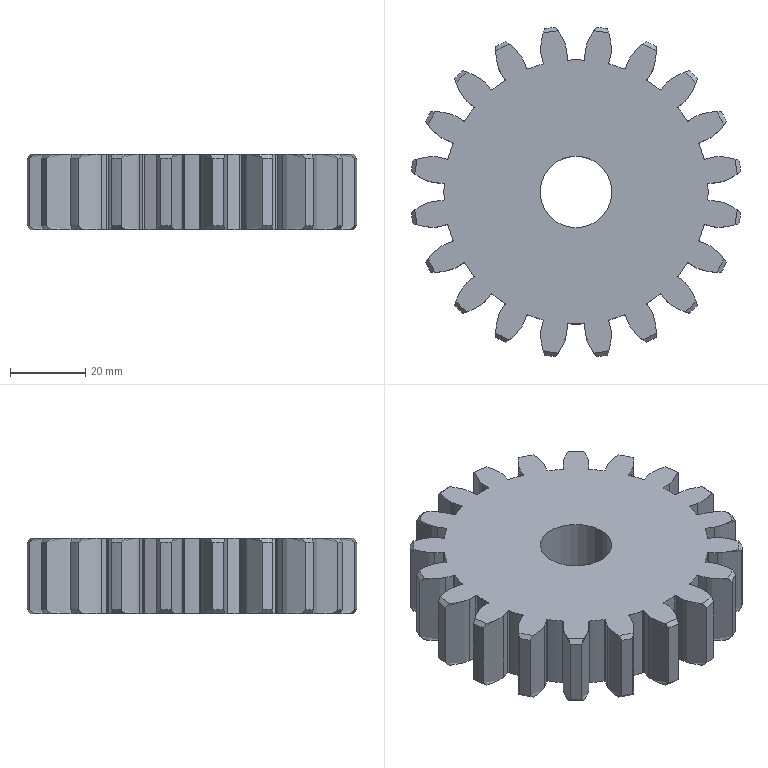Part | SolidWorks | 1 solid | 215 faces | box 87.341 x 87.341 x 20 mm | volume 92376 mm3 | cylinder 93 | plane 42 | cone 40 | spline 40 | commonest cylinder face diameters 0.6 x50 70 x21 88 x20 19 x2